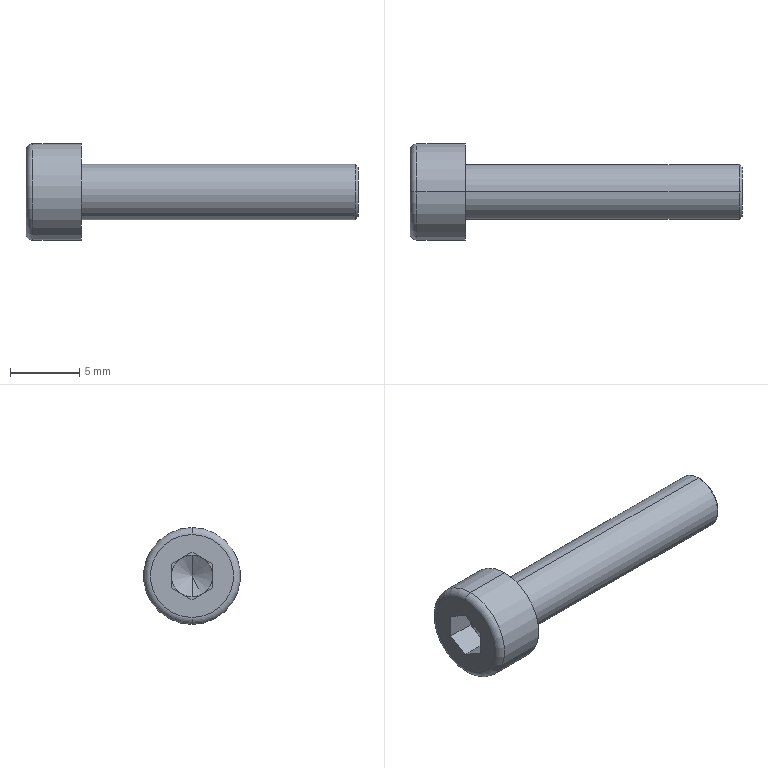Part | SolidWorks | features Fillet 2, RevCut 2, Boss 1, Chamfer 1, Cut 1, Extrusion 1, LPattern 1 | 1 solid | 25 faces | box 24 x 7 x 7 mm | volume 386.251 mm3 | plane 15 | cone 4 | cylinder 4 | torus 2 | commonest cylinder face diameters 4 x2 7 x2
STEP:
#1=CARTESIAN_POINT('',(24.,0.,-1.8));
#2=VERTEX_POINT('',#1);
#3=CARTESIAN_POINT('',(24.,0.,1.8));
#4=VERTEX_POINT('',#3);
#5=CARTESIAN_POINT('',(24.,0.,0.));
#6=DIRECTION('',(1.,0.,0.));
#7=DIRECTION('',(0.,0.,-1.));
#8=AXIS2_PLACEMENT_3D('',#5,#6,#7);
#9=CIRCLE('',#8,1.8);
#10=EDGE_CURVE('',#2,#4,#9,.T.);
#11=ORIENTED_EDGE('',*,*,#10,.F.);
#12=CARTESIAN_POINT('',(23.8,0.,-2.));
#13=VERTEX_POINT('',#12);
#14=CARTESIAN_POINT('',(24.,0.,-1.8));
#15=DIRECTION('',(-0.7071,0.,-0.7071));
#16=VECTOR('',#15,1000.);
#17=LINE('',#14,#16);
#18=EDGE_CURVE('',#2,#13,#17,.T.);
#19=ORIENTED_EDGE('',*,*,#18,.T.);
#20=CARTESIAN_POINT('',(23.8,0.,2.));
#21=VERTEX_POINT('',#20);
#22=CARTESIAN_POINT('',(23.8,0.,0.));
#23=DIRECTION('',(-1.,0.,0.));
#24=DIRECTION('',(0.,0.,-1.));
#25=AXIS2_PLACEMENT_3D('',#22,#23,#24);
#26=CIRCLE('',#25,2.);
#27=EDGE_CURVE('',#21,#13,#26,.T.);
#28=ORIENTED_EDGE('',*,*,#27,.F.);
#29=CARTESIAN_POINT('',(24.,0.,1.8));
#30=DIRECTION('',(-0.7071,0.,0.7071));
#31=VECTOR('',#30,1000.);
#32=LINE('',#29,#31);
#33=EDGE_CURVE('',#4,#21,#32,.T.);
#34=ORIENTED_EDGE('',*,*,#33,.F.);
#35=EDGE_LOOP('',(#11,#19,#28,#34));
#36=FACE_OUTER_BOUND('',#35,.T.);
#37=CARTESIAN_POINT('',(24.,0.,0.));
#38=DIRECTION('',(-1.,0.,0.));
#39=DIRECTION('',(0.,0.,1.));
#40=AXIS2_PLACEMENT_3D('',#37,#38,#39);
#41=CONICAL_SURFACE('',#40,1.8,0.7854);
#42=ADVANCED_FACE('',(#36),#41,.T.);
#43=CARTESIAN_POINT('',(0.,0.,3.));
#44=VERTEX_POINT('',#43);
#45=CARTESIAN_POINT('',(0.,0.,-3.));
#46=VERTEX_POINT('',#45);
#47=CARTESIAN_POINT('',(0.,0.,0.));
#48=DIRECTION('',(-1.,0.,0.));
#49=DIRECTION('',(0.,0.,-1.));
#50=AXIS2_PLACEMENT_3D('',#47,#48,#49);
#51=CIRCLE('',#50,3.);
#52=EDGE_CURVE('',#44,#46,#51,.T.);
#53=ORIENTED_EDGE('',*,*,#52,.F.);
#54=CARTESIAN_POINT('',(0.5,0.,3.5));
#55=VERTEX_POINT('',#54);
#56=CARTESIAN_POINT('',(0.5,0.,3.));
#57=DIRECTION('',(0.,1.,0.));
#58=DIRECTION('',(0.,0.,1.));
#59=AXIS2_PLACEMENT_3D('',#56,#57,#58);
#60=CIRCLE('',#59,0.5);
#61=EDGE_CURVE('',#44,#55,#60,.T.);
#62=ORIENTED_EDGE('',*,*,#61,.T.);
#63=CARTESIAN_POINT('',(0.5,0.,-3.5));
#64=VERTEX_POINT('',#63);
#65=CARTESIAN_POINT('',(0.5,0.,0.));
#66=DIRECTION('',(1.,0.,0.));
#67=DIRECTION('',(0.,0.,-1.));
#68=AXIS2_PLACEMENT_3D('',#65,#66,#67);
#69=CIRCLE('',#68,3.5);
#70=EDGE_CURVE('',#64,#55,#69,.T.);
#71=ORIENTED_EDGE('',*,*,#70,.F.);
#72=CARTESIAN_POINT('',(0.5,0.,-3.));
#73=DIRECTION('',(0.,-1.,0.));
#74=DIRECTION('',(0.,0.,-1.));
#75=AXIS2_PLACEMENT_3D('',#72,#73,#74);
#76=CIRCLE('',#75,0.5);
#77=EDGE_CURVE('',#46,#64,#76,.T.);
#78=ORIENTED_EDGE('',*,*,#77,.F.);
#79=EDGE_LOOP('',(#53,#62,#71,#78));
#80=FACE_OUTER_BOUND('',#79,.T.);
#81=CARTESIAN_POINT('',(0.5,0.,0.));
#82=DIRECTION('',(1.,0.,0.));
#83=DIRECTION('',(0.,0.,-1.));
#84=AXIS2_PLACEMENT_3D('',#81,#82,#83);
#85=TOROIDAL_SURFACE('',#84,3.,0.5);
#86=ADVANCED_FACE('',(#80),#85,.T.);
#87=CARTESIAN_POINT('',(2.866,0.,0.));
#88=VERTEX_POINT('',#87);
#89=CARTESIAN_POINT('',(2.,0.,1.5));
#90=VERTEX_POINT('',#89);
#91=CARTESIAN_POINT('',(2.,0.,1.5));
#92=DIRECTION('',(-0.5,0.,0.866));
#93=VECTOR('',#92,1000.);
#94=LINE('',#91,#93);
#95=EDGE_CURVE('',#88,#90,#94,.T.);
#96=ORIENTED_EDGE('',*,*,#95,.F.);
#97=CARTESIAN_POINT('',(2.,0.,-1.5));
#98=VERTEX_POINT('',#97);
#99=CARTESIAN_POINT('',(2.,0.,-1.5));
#100=DIRECTION('',(-0.5,0.,-0.866));
#101=VECTOR('',#100,1000.);
#102=LINE('',#99,#101);
#103=EDGE_CURVE('',#88,#98,#102,.T.);
#104=ORIENTED_EDGE('',*,*,#103,.T.);
#105=CARTESIAN_POINT('',(2.,-0.75,-1.299));
#106=VERTEX_POINT('',#105);
#107=CARTESIAN_POINT('',(2.,0.,0.));
#108=DIRECTION('',(1.,0.,0.));
#109=DIRECTION('',(0.,0.,1.));
#110=AXIS2_PLACEMENT_3D('',#107,#108,#109);
#111=CIRCLE('',#110,1.5);
#112=EDGE_CURVE('',#106,#98,#111,.T.);
#113=ORIENTED_EDGE('',*,*,#112,.F.);
#114=CARTESIAN_POINT('',(2.,-1.5,0.));
#115=VERTEX_POINT('',#114);
#116=CARTESIAN_POINT('',(2.,0.,0.));
#117=DIRECTION('',(1.,0.,0.));
#118=DIRECTION('',(0.,0.,1.));
#119=AXIS2_PLACEMENT_3D('',#116,#117,#118);
#120=CIRCLE('',#119,1.5);
#121=EDGE_CURVE('',#115,#106,#120,.T.);
#122=ORIENTED_EDGE('',*,*,#121,.F.);
#123=CARTESIAN_POINT('',(2.,-0.75,1.299));
#124=VERTEX_POINT('',#123);
#125=CARTESIAN_POINT('',(2.,0.,0.));
#126=DIRECTION('',(1.,0.,0.));
#127=DIRECTION('',(0.,0.,1.));
#128=AXIS2_PLACEMENT_3D('',#125,#126,#127);
#129=CIRCLE('',#128,1.5);
#130=EDGE_CURVE('',#124,#115,#129,.T.);
#131=ORIENTED_EDGE('',*,*,#130,.F.);
#132=CARTESIAN_POINT('',(2.,0.,0.));
#133=DIRECTION('',(1.,0.,0.));
#134=DIRECTION('',(0.,0.,1.));
#135=AXIS2_PLACEMENT_3D('',#132,#133,#134);
#136=CIRCLE('',#135,1.5);
#137=EDGE_CURVE('',#90,#124,#136,.T.);
#138=ORIENTED_EDGE('',*,*,#137,.F.);
#139=EDGE_LOOP('',(#96,#104,#113,#122,#131,#138));
#140=FACE_OUTER_BOUND('',#139,.T.);
#141=CARTESIAN_POINT('',(2.,0.,0.));
#142=DIRECTION('',(-1.,0.,0.));
#143=DIRECTION('',(0.,0.,1.));
#144=AXIS2_PLACEMENT_3D('',#141,#142,#143);
#145=CONICAL_SURFACE('',#144,1.5,1.047);
#146=ADVANCED_FACE('',(#140),#145,.F.);
#147=ORIENTED_EDGE('',*,*,#27,.T.);
#148=CARTESIAN_POINT('',(4.,0.,-2.));
#149=VERTEX_POINT('',#148);
#150=CARTESIAN_POINT('',(24.,0.,-2.));
#151=DIRECTION('',(-1.,0.,0.));
#152=VECTOR('',#151,1000.);
#153=LINE('',#150,#152);
#154=EDGE_CURVE('',#13,#149,#153,.T.);
#155=ORIENTED_EDGE('',*,*,#154,.T.);
#156=CARTESIAN_POINT('',(4.,0.,2.));
#157=VERTEX_POINT('',#156);
#158=CARTESIAN_POINT('',(4.,0.,0.));
#159=DIRECTION('',(1.,0.,0.));
#160=DIRECTION('',(0.,0.,-1.));
#161=AXIS2_PLACEMENT_3D('',#158,#159,#160);
#162=CIRCLE('',#161,2.);
#163=EDGE_CURVE('',#149,#157,#162,.T.);
#164=ORIENTED_EDGE('',*,*,#163,.T.);
#165=CARTESIAN_POINT('',(24.,0.,2.));
#166=DIRECTION('',(-1.,0.,0.));
#167=VECTOR('',#166,1000.);
#168=LINE('',#165,#167);
#169=EDGE_CURVE('',#21,#157,#168,.T.);
#170=ORIENTED_EDGE('',*,*,#169,.F.);
#171=EDGE_LOOP('',(#147,#155,#164,#170));
#172=FACE_OUTER_BOUND('',#171,.T.);
#173=CARTESIAN_POINT('',(24.,0.,0.));
#174=DIRECTION('',(-1.,0.,0.));
#175=DIRECTION('',(0.,0.,1.));
#176=AXIS2_PLACEMENT_3D('',#173,#174,#175);
#177=CYLINDRICAL_SURFACE('',#176,2.);
#178=ADVANCED_FACE('',(#172),#177,.T.);
#179=CARTESIAN_POINT('',(4.,0.,-3.5));
#180=VERTEX_POINT('',#179);
#181=CARTESIAN_POINT('',(4.,0.,3.5));
#182=VERTEX_POINT('',#181);
#183=CARTESIAN_POINT('',(4.,0.,0.));
#184=DIRECTION('',(1.,0.,0.));
#185=DIRECTION('',(0.,0.,-1.));
#186=AXIS2_PLACEMENT_3D('',#183,#184,#185);
#187=CIRCLE('',#186,3.5);
#188=EDGE_CURVE('',#180,#182,#187,.T.);
#189=ORIENTED_EDGE('',*,*,#188,.F.);
#190=CARTESIAN_POINT('',(4.,0.,-3.5));
#191=DIRECTION('',(-1.,0.,0.));
#192=VECTOR('',#191,1000.);
#193=LINE('',#190,#192);
#194=EDGE_CURVE('',#180,#64,#193,.T.);
#195=ORIENTED_EDGE('',*,*,#194,.T.);
#196=ORIENTED_EDGE('',*,*,#70,.T.);
#197=CARTESIAN_POINT('',(4.,0.,3.5));
#198=DIRECTION('',(-1.,0.,0.));
#199=VECTOR('',#198,1000.);
#200=LINE('',#197,#199);
#201=EDGE_CURVE('',#182,#55,#200,.T.);
#202=ORIENTED_EDGE('',*,*,#201,.F.);
#203=EDGE_LOOP('',(#189,#195,#196,#202));
#204=FACE_OUTER_BOUND('',#203,.T.);
#205=CARTESIAN_POINT('',(4.,0.,0.));
#206=DIRECTION('',(-1.,0.,0.));
#207=DIRECTION('',(0.,0.,1.));
#208=AXIS2_PLACEMENT_3D('',#205,#206,#207);
#209=CYLINDRICAL_SURFACE('',#208,3.5);
#210=ADVANCED_FACE('',(#204),#209,.T.);
#211=CARTESIAN_POINT('',(2.,-1.5,0.866));
#212=VERTEX_POINT('',#211);
#213=CARTESIAN_POINT('',(2.,0.,1.732));
#214=DIRECTION('',(0.,-0.866,-0.5));
#215=VECTOR('',#214,1000.);
#216=LINE('',#213,#215);
#217=EDGE_CURVE('',#124,#212,#216,.T.);
#218=ORIENTED_EDGE('',*,*,#217,.F.);
#219=ORIENTED_EDGE('',*,*,#130,.T.);
#220=CARTESIAN_POINT('',(2.,-1.5,0.866));
#221=DIRECTION('',(0.,0.,-1.));
#222=VECTOR('',#221,1000.);
#223=LINE('',#220,#222);
#224=EDGE_CURVE('',#212,#115,#223,.T.);
#225=ORIENTED_EDGE('',*,*,#224,.F.);
#226=EDGE_LOOP('',(#218,#219,#225));
#227=FACE_OUTER_BOUND('',#226,.T.);
#228=CARTESIAN_POINT('',(2.,-3.,0.));
#229=DIRECTION('',(-1.,0.,0.));
#230=DIRECTION('',(0.,0.,1.));
#231=AXIS2_PLACEMENT_3D('',#228,#229,#230);
#232=PLANE('',#231);
#233=ADVANCED_FACE('',(#227),#232,.T.);
#234=CARTESIAN_POINT('',(2.,-1.5,-0.866));
#235=VERTEX_POINT('',#234);
#236=CARTESIAN_POINT('',(2.,-1.5,0.866));
#237=DIRECTION('',(0.,0.,-1.));
#238=VECTOR('',#237,1000.);
#239=LINE('',#236,#238);
#240=EDGE_CURVE('',#115,#235,#239,.T.);
#241=ORIENTED_EDGE('',*,*,#240,.F.);
#242=ORIENTED_EDGE('',*,*,#121,.T.);
#243=CARTESIAN_POINT('',(2.,-1.5,-0.866));
#244=DIRECTION('',(0.,0.866,-0.5));
#245=VECTOR('',#244,1000.);
#246=LINE('',#243,#245);
#247=EDGE_CURVE('',#235,#106,#246,.T.);
#248=ORIENTED_EDGE('',*,*,#247,.F.);
#249=EDGE_LOOP('',(#241,#242,#248));
#250=FACE_OUTER_BOUND('',#249,.T.);
#251=CARTESIAN_POINT('',(2.,-3.,0.));
#252=DIRECTION('',(-1.,0.,0.));
#253=DIRECTION('',(0.,0.,1.));
#254=AXIS2_PLACEMENT_3D('',#251,#252,#253);
#255=PLANE('',#254);
#256=ADVANCED_FACE('',(#250),#255,.T.);
#257=CARTESIAN_POINT('',(2.,0.,-1.732));
#258=VERTEX_POINT('',#257);
#259=CARTESIAN_POINT('',(2.,-1.5,-0.866));
#260=DIRECTION('',(0.,0.866,-0.5));
#261=VECTOR('',#260,1000.);
#262=LINE('',#259,#261);
#263=EDGE_CURVE('',#106,#258,#262,.T.);
#264=ORIENTED_EDGE('',*,*,#263,.F.);
#265=ORIENTED_EDGE('',*,*,#112,.T.);
#266=CARTESIAN_POINT('',(2.,0.75,-1.299));
#267=VERTEX_POINT('',#266);
#268=CARTESIAN_POINT('',(2.,0.,0.));
#269=DIRECTION('',(1.,0.,0.));
#270=DIRECTION('',(0.,0.,1.));
#271=AXIS2_PLACEMENT_3D('',#268,#269,#270);
#272=CIRCLE('',#271,1.5);
#273=EDGE_CURVE('',#98,#267,#272,.T.);
#274=ORIENTED_EDGE('',*,*,#273,.T.);
#275=CARTESIAN_POINT('',(2.,0.,-1.732));
#276=DIRECTION('',(0.,0.866,0.5));
#277=VECTOR('',#276,1000.);
#278=LINE('',#275,#277);
#279=EDGE_CURVE('',#258,#267,#278,.T.);
#280=ORIENTED_EDGE('',*,*,#279,.F.);
#281=EDGE_LOOP('',(#264,#265,#274,#280));
#282=FACE_OUTER_BOUND('',#281,.T.);
#283=CARTESIAN_POINT('',(2.,-3.,0.));
#284=DIRECTION('',(-1.,0.,0.));
#285=DIRECTION('',(0.,0.,1.));
#286=AXIS2_PLACEMENT_3D('',#283,#284,#285);
#287=PLANE('',#286);
#288=ADVANCED_FACE('',(#282),#287,.T.);
#289=CARTESIAN_POINT('',(2.,1.5,-0.866));
#290=VERTEX_POINT('',#289);
#291=CARTESIAN_POINT('',(2.,0.,-1.732));
#292=DIRECTION('',(0.,0.866,0.5));
#293=VECTOR('',#292,1000.);
#294=LINE('',#291,#293);
#295=EDGE_CURVE('',#267,#290,#294,.T.);
#296=ORIENTED_EDGE('',*,*,#295,.F.);
#297=CARTESIAN_POINT('',(2.,1.5,0.));
#298=VERTEX_POINT('',#297);
#299=CARTESIAN_POINT('',(2.,0.,0.));
#300=DIRECTION('',(1.,0.,0.));
#301=DIRECTION('',(0.,0.,-1.));
#302=AXIS2_PLACEMENT_3D('',#299,#300,#301);
#303=CIRCLE('',#302,1.5);
#304=EDGE_CURVE('',#267,#298,#303,.T.);
#305=ORIENTED_EDGE('',*,*,#304,.T.);
#306=CARTESIAN_POINT('',(2.,1.5,-0.866));
#307=DIRECTION('',(0.,0.,1.));
#308=VECTOR('',#307,1000.);
#309=LINE('',#306,#308);
#310=EDGE_CURVE('',#290,#298,#309,.T.);
#311=ORIENTED_EDGE('',*,*,#310,.F.);
#312=EDGE_LOOP('',(#296,#305,#311));
#313=FACE_OUTER_BOUND('',#312,.T.);
#314=CARTESIAN_POINT('',(2.,-3.,0.));
#315=DIRECTION('',(-1.,0.,0.));
#316=DIRECTION('',(0.,0.,1.));
#317=AXIS2_PLACEMENT_3D('',#314,#315,#316);
#318=PLANE('',#317);
#319=ADVANCED_FACE('',(#313),#318,.T.);
#320=CARTESIAN_POINT('',(2.,1.5,0.866));
#321=VERTEX_POINT('',#320);
#322=CARTESIAN_POINT('',(2.,1.5,-0.866));
#323=DIRECTION('',(0.,0.,1.));
#324=VECTOR('',#323,1000.);
#325=LINE('',#322,#324);
#326=EDGE_CURVE('',#298,#321,#325,.T.);
#327=ORIENTED_EDGE('',*,*,#326,.F.);
#328=CARTESIAN_POINT('',(2.,0.75,1.299));
#329=VERTEX_POINT('',#328);
#330=CARTESIAN_POINT('',(2.,0.,0.));
#331=DIRECTION('',(1.,0.,0.));
#332=DIRECTION('',(0.,0.,1.));
#333=AXIS2_PLACEMENT_3D('',#330,#331,#332);
#334=CIRCLE('',#333,1.5);
#335=EDGE_CURVE('',#298,#329,#334,.T.);
#336=ORIENTED_EDGE('',*,*,#335,.T.);
#337=CARTESIAN_POINT('',(2.,1.5,0.866));
#338=DIRECTION('',(0.,-0.866,0.5));
#339=VECTOR('',#338,1000.);
#340=LINE('',#337,#339);
#341=EDGE_CURVE('',#321,#329,#340,.T.);
#342=ORIENTED_EDGE('',*,*,#341,.F.);
#343=EDGE_LOOP('',(#327,#336,#342));
#344=FACE_OUTER_BOUND('',#343,.T.);
#345=CARTESIAN_POINT('',(2.,-3.,0.));
#346=DIRECTION('',(-1.,0.,0.));
#347=DIRECTION('',(0.,0.,1.));
#348=AXIS2_PLACEMENT_3D('',#345,#346,#347);
#349=PLANE('',#348);
#350=ADVANCED_FACE('',(#344),#349,.T.);
#351=CARTESIAN_POINT('',(2.,0.,1.732));
#352=VERTEX_POINT('',#351);
#353=CARTESIAN_POINT('',(2.,1.5,0.866));
#354=DIRECTION('',(0.,-0.866,0.5));
#355=VECTOR('',#354,1000.);
#356=LINE('',#353,#355);
#357=EDGE_CURVE('',#329,#352,#356,.T.);
#358=ORIENTED_EDGE('',*,*,#357,.F.);
#359=CARTESIAN_POINT('',(2.,0.,0.));
#360=DIRECTION('',(1.,0.,0.));
#361=DIRECTION('',(0.,0.,1.));
#362=AXIS2_PLACEMENT_3D('',#359,#360,#361);
#363=CIRCLE('',#362,1.5);
#364=EDGE_CURVE('',#329,#90,#363,.T.);
#365=ORIENTED_EDGE('',*,*,#364,.T.);
#366=ORIENTED_EDGE('',*,*,#137,.T.);
#367=CARTESIAN_POINT('',(2.,0.,1.732));
#368=DIRECTION('',(0.,-0.866,-0.5));
#369=VECTOR('',#368,1000.);
#370=LINE('',#367,#369);
#371=EDGE_CURVE('',#352,#124,#370,.T.);
#372=ORIENTED_EDGE('',*,*,#371,.F.);
#373=EDGE_LOOP('',(#358,#365,#366,#372));
#374=FACE_OUTER_BOUND('',#373,.T.);
#375=CARTESIAN_POINT('',(2.,-3.,0.));
#376=DIRECTION('',(-1.,0.,0.));
#377=DIRECTION('',(0.,0.,1.));
#378=AXIS2_PLACEMENT_3D('',#375,#376,#377);
#379=PLANE('',#378);
#380=ADVANCED_FACE('',(#374),#379,.T.);
#381=CARTESIAN_POINT('',(0.,0.,0.));
#382=DIRECTION('',(-1.,0.,0.));
#383=DIRECTION('',(0.,0.,-1.));
#384=AXIS2_PLACEMENT_3D('',#381,#382,#383);
#385=CIRCLE('',#384,3.);
#386=EDGE_CURVE('',#46,#44,#385,.T.);
#387=ORIENTED_EDGE('',*,*,#386,.T.);
#388=ORIENTED_EDGE('',*,*,#52,.T.);
#389=EDGE_LOOP('',(#387,#388));
#390=FACE_OUTER_BOUND('',#389,.T.);
#391=CARTESIAN_POINT('',(0.,-1.5,-0.866));
#392=VERTEX_POINT('',#391);
#393=CARTESIAN_POINT('',(0.,0.,-1.732));
#394=VERTEX_POINT('',#393);
#395=CARTESIAN_POINT('',(0.,-1.5,-0.866));
#396=DIRECTION('',(0.,0.866,-0.5));
#397=VECTOR('',#396,1000.);
#398=LINE('',#395,#397);
#399=EDGE_CURVE('',#392,#394,#398,.T.);
#400=ORIENTED_EDGE('',*,*,#399,.T.);
#401=CARTESIAN_POINT('',(0.,1.5,-0.866));
#402=VERTEX_POINT('',#401);
#403=CARTESIAN_POINT('',(0.,0.,-1.732));
#404=DIRECTION('',(0.,0.866,0.5));
#405=VECTOR('',#404,1000.);
#406=LINE('',#403,#405);
#407=EDGE_CURVE('',#394,#402,#406,.T.);
#408=ORIENTED_EDGE('',*,*,#407,.T.);
#409=CARTESIAN_POINT('',(0.,1.5,0.866));
#410=VERTEX_POINT('',#409);
#411=CARTESIAN_POINT('',(0.,1.5,-0.866));
#412=DIRECTION('',(0.,0.,1.));
#413=VECTOR('',#412,1000.);
#414=LINE('',#411,#413);
#415=EDGE_CURVE('',#402,#410,#414,.T.);
#416=ORIENTED_EDGE('',*,*,#415,.T.);
#417=CARTESIAN_POINT('',(0.,0.,1.732));
#418=VERTEX_POINT('',#417);
#419=CARTESIAN_POINT('',(0.,1.5,0.866));
#420=DIRECTION('',(0.,-0.866,0.5));
#421=VECTOR('',#420,1000.);
#422=LINE('',#419,#421);
#423=EDGE_CURVE('',#410,#418,#422,.T.);
#424=ORIENTED_EDGE('',*,*,#423,.T.);
#425=CARTESIAN_POINT('',(0.,-1.5,0.866));
#426=VERTEX_POINT('',#425);
#427=CARTESIAN_POINT('',(0.,0.,1.732));
#428=DIRECTION('',(0.,-0.866,-0.5));
#429=VECTOR('',#428,1000.);
#430=LINE('',#427,#429);
#431=EDGE_CURVE('',#418,#426,#430,.T.);
#432=ORIENTED_EDGE('',*,*,#431,.T.);
#433=CARTESIAN_POINT('',(0.,-1.5,0.866));
#434=DIRECTION('',(0.,0.,-1.));
#435=VECTOR('',#434,1000.);
#436=LINE('',#433,#435);
#437=EDGE_CURVE('',#426,#392,#436,.T.);
#438=ORIENTED_EDGE('',*,*,#437,.T.);
#439=EDGE_LOOP('',(#400,#408,#416,#424,#432,#438));
#440=FACE_BOUND('',#439,.T.);
#441=CARTESIAN_POINT('',(0.,0.,0.));
#442=DIRECTION('',(1.,0.,0.));
#443=DIRECTION('',(0.,0.,-1.));
#444=AXIS2_PLACEMENT_3D('',#441,#442,#443);
#445=PLANE('',#444);
#446=ADVANCED_FACE('',(#390,#440),#445,.F.);
#447=CARTESIAN_POINT('',(4.,0.,0.));
#448=DIRECTION('',(1.,0.,0.));
#449=DIRECTION('',(0.,0.,-1.));
#450=AXIS2_PLACEMENT_3D('',#447,#448,#449);
#451=CIRCLE('',#450,3.5);
#452=EDGE_CURVE('',#182,#180,#451,.T.);
#453=ORIENTED_EDGE('',*,*,#452,.T.);
#454=ORIENTED_EDGE('',*,*,#188,.T.);
#455=EDGE_LOOP('',(#453,#454));
#456=FACE_OUTER_BOUND('',#455,.T.);
#457=CARTESIAN_POINT('',(4.,0.,0.));
#458=DIRECTION('',(1.,0.,0.));
#459=DIRECTION('',(0.,0.,-1.));
#460=AXIS2_PLACEMENT_3D('',#457,#458,#459);
#461=CIRCLE('',#460,2.);
#462=EDGE_CURVE('',#157,#149,#461,.T.);
#463=ORIENTED_EDGE('',*,*,#462,.F.);
#464=ORIENTED_EDGE('',*,*,#163,.F.);
#465=EDGE_LOOP('',(#463,#464));
#466=FACE_BOUND('',#465,.T.);
#467=CARTESIAN_POINT('',(4.,0.,0.));
#468=DIRECTION('',(1.,0.,0.));
#469=DIRECTION('',(0.,0.,-1.));
#470=AXIS2_PLACEMENT_3D('',#467,#468,#469);
#471=PLANE('',#470);
#472=ADVANCED_FACE('',(#456,#466),#471,.T.);
#473=ORIENTED_EDGE('',*,*,#194,.F.);
#474=ORIENTED_EDGE('',*,*,#452,.F.);
#475=ORIENTED_EDGE('',*,*,#201,.T.);
#476=CARTESIAN_POINT('',(0.5,0.,0.));
#477=DIRECTION('',(1.,0.,0.));
#478=DIRECTION('',(0.,0.,-1.));
#479=AXIS2_PLACEMENT_3D('',#476,#477,#478);
#480=CIRCLE('',#479,3.5);
#481=EDGE_CURVE('',#55,#64,#480,.T.);
#482=ORIENTED_EDGE('',*,*,#481,.T.);
#483=EDGE_LOOP('',(#473,#474,#475,#482));
#484=FACE_OUTER_BOUND('',#483,.T.);
#485=CARTESIAN_POINT('',(4.,0.,0.));
#486=DIRECTION('',(-1.,0.,0.));
#487=DIRECTION('',(0.,0.,1.));
#488=AXIS2_PLACEMENT_3D('',#485,#486,#487);
#489=CYLINDRICAL_SURFACE('',#488,3.5);
#490=ADVANCED_FACE('',(#484),#489,.T.);
#491=ORIENTED_EDGE('',*,*,#154,.F.);
#492=CARTESIAN_POINT('',(23.8,0.,0.));
#493=DIRECTION('',(-1.,0.,0.));
#494=DIRECTION('',(0.,0.,-1.));
#495=AXIS2_PLACEMENT_3D('',#492,#493,#494);
#496=CIRCLE('',#495,2.);
#497=EDGE_CURVE('',#13,#21,#496,.T.);
#498=ORIENTED_EDGE('',*,*,#497,.T.);
#499=ORIENTED_EDGE('',*,*,#169,.T.);
#500=ORIENTED_EDGE('',*,*,#462,.T.);
#501=EDGE_LOOP('',(#491,#498,#499,#500));
#502=FACE_OUTER_BOUND('',#501,.T.);
#503=CARTESIAN_POINT('',(24.,0.,0.));
#504=DIRECTION('',(-1.,0.,0.));
#505=DIRECTION('',(0.,0.,1.));
#506=AXIS2_PLACEMENT_3D('',#503,#504,#505);
#507=CYLINDRICAL_SURFACE('',#506,2.);
#508=ADVANCED_FACE('',(#502),#507,.T.);
#509=CARTESIAN_POINT('',(24.,0.,0.));
#510=DIRECTION('',(1.,0.,0.));
#511=DIRECTION('',(0.,0.,-1.));
#512=AXIS2_PLACEMENT_3D('',#509,#510,#511);
#513=CIRCLE('',#512,1.8);
#514=EDGE_CURVE('',#4,#2,#513,.T.);
#515=ORIENTED_EDGE('',*,*,#514,.T.);
#516=ORIENTED_EDGE('',*,*,#10,.T.);
#517=EDGE_LOOP('',(#515,#516));
#518=FACE_OUTER_BOUND('',#517,.T.);
#519=CARTESIAN_POINT('',(24.,0.,0.));
#520=DIRECTION('',(1.,0.,0.));
#521=DIRECTION('',(0.,0.,-1.));
#522=AXIS2_PLACEMENT_3D('',#519,#520,#521);
#523=PLANE('',#522);
#524=ADVANCED_FACE('',(#518),#523,.T.);
#525=ORIENTED_EDGE('',*,*,#399,.F.);
#526=CARTESIAN_POINT('',(2.,-1.5,-0.866));
#527=DIRECTION('',(-1.,0.,0.));
#528=VECTOR('',#527,1000.);
#529=LINE('',#526,#528);
#530=EDGE_CURVE('',#235,#392,#529,.T.);
#531=ORIENTED_EDGE('',*,*,#530,.F.);
#532=ORIENTED_EDGE('',*,*,#247,.T.);
#533=ORIENTED_EDGE('',*,*,#263,.T.);
#534=CARTESIAN_POINT('',(2.,0.,-1.732));
#535=DIRECTION('',(-1.,0.,0.));
#536=VECTOR('',#535,1000.);
#537=LINE('',#534,#536);
#538=EDGE_CURVE('',#258,#394,#537,.T.);
#539=ORIENTED_EDGE('',*,*,#538,.T.);
#540=EDGE_LOOP('',(#525,#531,#532,#533,#539));
#541=FACE_OUTER_BOUND('',#540,.T.);
#542=CARTESIAN_POINT('',(2.,-1.5,-0.866));
#543=DIRECTION('',(0.,0.5,0.866));
#544=DIRECTION('',(0.,-0.866,0.5));
#545=AXIS2_PLACEMENT_3D('',#542,#543,#544);
#546=PLANE('',#545);
#547=ADVANCED_FACE('',(#541),#546,.T.);
#548=ORIENTED_EDGE('',*,*,#407,.F.);
#549=ORIENTED_EDGE('',*,*,#538,.F.);
#550=ORIENTED_EDGE('',*,*,#279,.T.);
#551=ORIENTED_EDGE('',*,*,#295,.T.);
#552=CARTESIAN_POINT('',(2.,1.5,-0.866));
#553=DIRECTION('',(-1.,0.,0.));
#554=VECTOR('',#553,1000.);
#555=LINE('',#552,#554);
#556=EDGE_CURVE('',#290,#402,#555,.T.);
#557=ORIENTED_EDGE('',*,*,#556,.T.);
#558=EDGE_LOOP('',(#548,#549,#550,#551,#557));
#559=FACE_OUTER_BOUND('',#558,.T.);
#560=CARTESIAN_POINT('',(2.,0.,-1.732));
#561=DIRECTION('',(0.,-0.5,0.866));
#562=DIRECTION('',(0.,-0.866,-0.5));
#563=AXIS2_PLACEMENT_3D('',#560,#561,#562);
#564=PLANE('',#563);
#565=ADVANCED_FACE('',(#559),#564,.T.);
#566=ORIENTED_EDGE('',*,*,#415,.F.);
#567=ORIENTED_EDGE('',*,*,#556,.F.);
#568=ORIENTED_EDGE('',*,*,#310,.T.);
#569=ORIENTED_EDGE('',*,*,#326,.T.);
#570=CARTESIAN_POINT('',(2.,1.5,0.866));
#571=DIRECTION('',(-1.,0.,0.));
#572=VECTOR('',#571,1000.);
#573=LINE('',#570,#572);
#574=EDGE_CURVE('',#321,#410,#573,.T.);
#575=ORIENTED_EDGE('',*,*,#574,.T.);
#576=EDGE_LOOP('',(#566,#567,#568,#569,#575));
#577=FACE_OUTER_BOUND('',#576,.T.);
#578=CARTESIAN_POINT('',(2.,1.5,-0.866));
#579=DIRECTION('',(0.,-1.,0.));
#580=DIRECTION('',(0.,0.,-1.));
#581=AXIS2_PLACEMENT_3D('',#578,#579,#580);
#582=PLANE('',#581);
#583=ADVANCED_FACE('',(#577),#582,.T.);
#584=ORIENTED_EDGE('',*,*,#423,.F.);
#585=ORIENTED_EDGE('',*,*,#574,.F.);
#586=ORIENTED_EDGE('',*,*,#341,.T.);
#587=ORIENTED_EDGE('',*,*,#357,.T.);
#588=CARTESIAN_POINT('',(2.,0.,1.732));
#589=DIRECTION('',(-1.,0.,0.));
#590=VECTOR('',#589,1000.);
#591=LINE('',#588,#590);
#592=EDGE_CURVE('',#352,#418,#591,.T.);
#593=ORIENTED_EDGE('',*,*,#592,.T.);
#594=EDGE_LOOP('',(#584,#585,#586,#587,#593));
#595=FACE_OUTER_BOUND('',#594,.T.);
#596=CARTESIAN_POINT('',(2.,1.5,0.866));
#597=DIRECTION('',(0.,-0.5,-0.866));
#598=DIRECTION('',(0.,0.866,-0.5));
#599=AXIS2_PLACEMENT_3D('',#596,#597,#598);
#600=PLANE('',#599);
#601=ADVANCED_FACE('',(#595),#600,.T.);
#602=ORIENTED_EDGE('',*,*,#431,.F.);
#603=ORIENTED_EDGE('',*,*,#592,.F.);
#604=ORIENTED_EDGE('',*,*,#371,.T.);
#605=ORIENTED_EDGE('',*,*,#217,.T.);
#606=CARTESIAN_POINT('',(2.,-1.5,0.866));
#607=DIRECTION('',(-1.,0.,0.));
#608=VECTOR('',#607,1000.);
#609=LINE('',#606,#608);
#610=EDGE_CURVE('',#212,#426,#609,.T.);
#611=ORIENTED_EDGE('',*,*,#610,.T.);
#612=EDGE_LOOP('',(#602,#603,#604,#605,#611));
#613=FACE_OUTER_BOUND('',#612,.T.);
#614=CARTESIAN_POINT('',(2.,0.,1.732));
#615=DIRECTION('',(0.,0.5,-0.866));
#616=DIRECTION('',(0.,0.866,0.5));
#617=AXIS2_PLACEMENT_3D('',#614,#615,#616);
#618=PLANE('',#617);
#619=ADVANCED_FACE('',(#613),#618,.T.);
#620=ORIENTED_EDGE('',*,*,#437,.F.);
#621=ORIENTED_EDGE('',*,*,#610,.F.);
#622=ORIENTED_EDGE('',*,*,#224,.T.);
#623=ORIENTED_EDGE('',*,*,#240,.T.);
#624=ORIENTED_EDGE('',*,*,#530,.T.);
#625=EDGE_LOOP('',(#620,#621,#622,#623,#624));
#626=FACE_OUTER_BOUND('',#625,.T.);
#627=CARTESIAN_POINT('',(2.,-1.5,0.866));
#628=DIRECTION('',(0.,1.,0.));
#629=DIRECTION('',(0.,0.,1.));
#630=AXIS2_PLACEMENT_3D('',#627,#628,#629);
#631=PLANE('',#630);
#632=ADVANCED_FACE('',(#626),#631,.T.);
#633=ORIENTED_EDGE('',*,*,#103,.F.);
#634=ORIENTED_EDGE('',*,*,#95,.T.);
#635=ORIENTED_EDGE('',*,*,#364,.F.);
#636=ORIENTED_EDGE('',*,*,#335,.F.);
#637=ORIENTED_EDGE('',*,*,#304,.F.);
#638=ORIENTED_EDGE('',*,*,#273,.F.);
#639=EDGE_LOOP('',(#633,#634,#635,#636,#637,#638));
#640=FACE_OUTER_BOUND('',#639,.T.);
#641=CARTESIAN_POINT('',(2.,0.,0.));
#642=DIRECTION('',(-1.,0.,0.));
#643=DIRECTION('',(0.,0.,1.));
#644=AXIS2_PLACEMENT_3D('',#641,#642,#643);
#645=CONICAL_SURFACE('',#644,1.5,1.047);
#646=ADVANCED_FACE('',(#640),#645,.F.);
#647=ORIENTED_EDGE('',*,*,#61,.F.);
#648=ORIENTED_EDGE('',*,*,#386,.F.);
#649=ORIENTED_EDGE('',*,*,#77,.T.);
#650=ORIENTED_EDGE('',*,*,#481,.F.);
#651=EDGE_LOOP('',(#647,#648,#649,#650));
#652=FACE_OUTER_BOUND('',#651,.T.);
#653=CARTESIAN_POINT('',(0.5,0.,0.));
#654=DIRECTION('',(1.,0.,0.));
#655=DIRECTION('',(0.,0.,-1.));
#656=AXIS2_PLACEMENT_3D('',#653,#654,#655);
#657=TOROIDAL_SURFACE('',#656,3.,0.5);
#658=ADVANCED_FACE('',(#652),#657,.T.);
#659=ORIENTED_EDGE('',*,*,#18,.F.);
#660=ORIENTED_EDGE('',*,*,#514,.F.);
#661=ORIENTED_EDGE('',*,*,#33,.T.);
#662=ORIENTED_EDGE('',*,*,#497,.F.);
#663=EDGE_LOOP('',(#659,#660,#661,#662));
#664=FACE_OUTER_BOUND('',#663,.T.);
#665=CARTESIAN_POINT('',(24.,0.,0.));
#666=DIRECTION('',(-1.,0.,0.));
#667=DIRECTION('',(0.,0.,1.));
#668=AXIS2_PLACEMENT_3D('',#665,#666,#667);
#669=CONICAL_SURFACE('',#668,1.8,0.7854);
#670=ADVANCED_FACE('',(#664),#669,.T.);
#671=CLOSED_SHELL('',(#42,#86,#146,#178,#210,#233,#256,#288,#319,#350,#380,#446,#472,#490,#508,#524,#547,#565,#583,#601,#619,#632,#646,#658,#670));
#672=MANIFOLD_SOLID_BREP('',#671);
#673=CARTESIAN_POINT('',(0.,0.,0.));
#674=DIRECTION('',(0.,0.,1.));
#675=DIRECTION('',(1.,0.,0.));
#676=AXIS2_PLACEMENT_3D('',#673,#674,#675);
#677=(LENGTH_UNIT()NAMED_UNIT(*)SI_UNIT(.MILLI.,.METRE.));
#678=UNCERTAINTY_MEASURE_WITH_UNIT(LENGTH_MEASURE(0.00001),#677,'','');
#679=(NAMED_UNIT(*)PLANE_ANGLE_UNIT()SI_UNIT($,.RADIAN.));
#680=(NAMED_UNIT(*)SI_UNIT($,.STERADIAN.)SOLID_ANGLE_UNIT());
#681=(GEOMETRIC_REPRESENTATION_CONTEXT(3)GLOBAL_UNCERTAINTY_ASSIGNED_CONTEXT((#678))GLOBAL_UNIT_ASSIGNED_CONTEXT((#677,#679,#680))REPRESENTATION_CONTEXT('',''));
#682=ADVANCED_BREP_SHAPE_REPRESENTATION('',(#672,#676),#681);